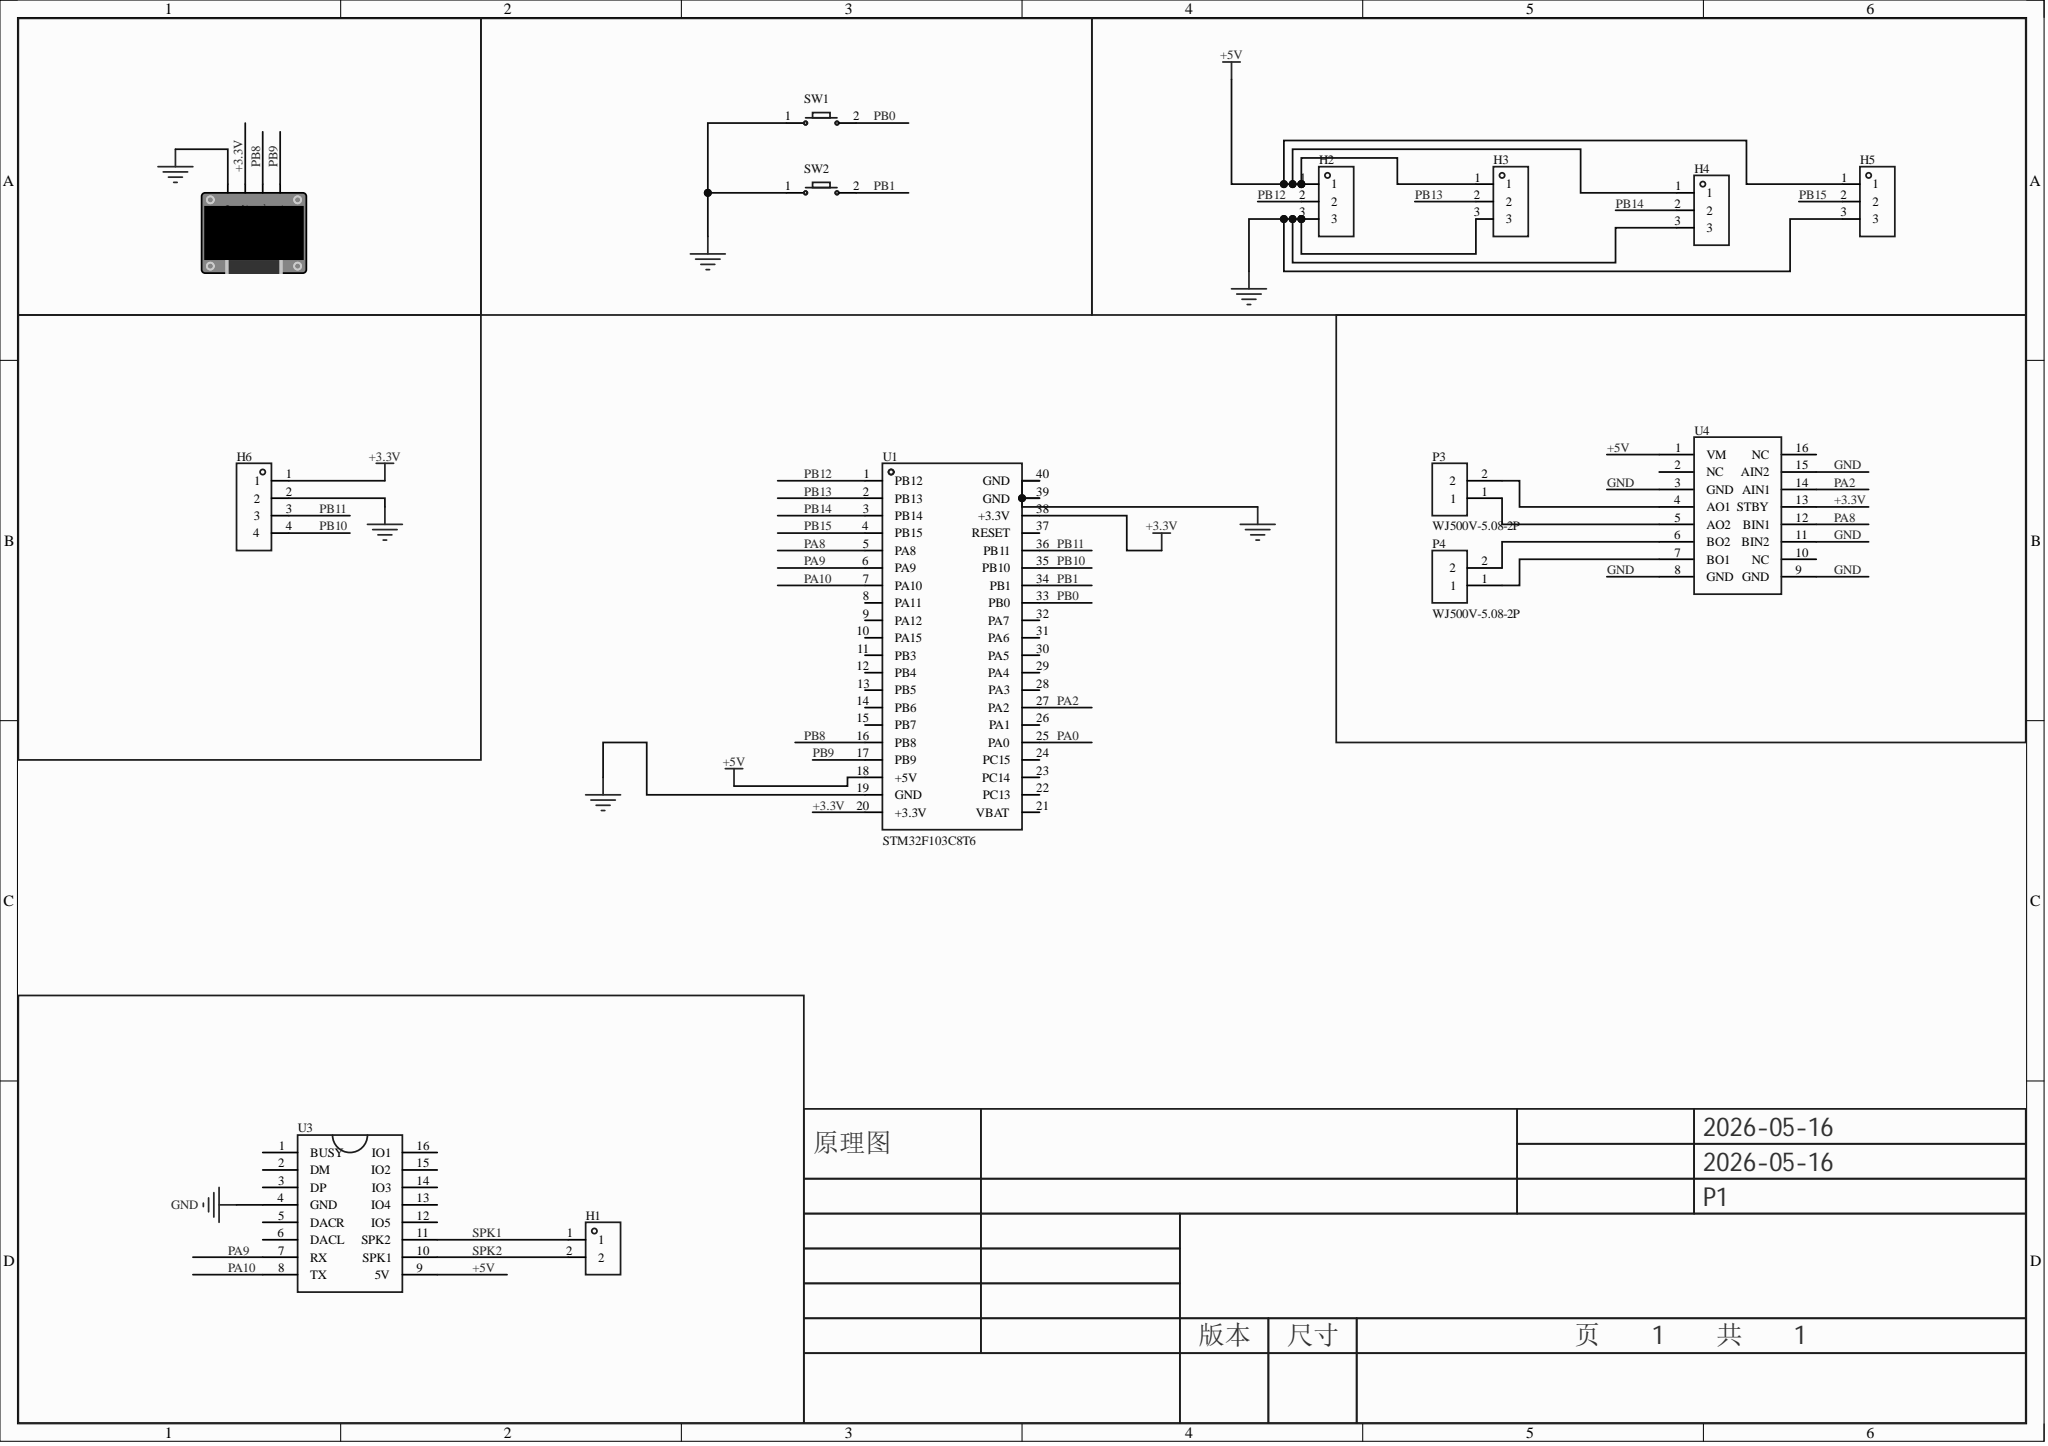Circuit board | Altium Designer | 14 parts | 23 nets
Bill of materials:
Comment,Description,Designator,Footprint,LibRef,Quantity
"HX PH254-01-02-Z-L11.5 male header connector","","H1","HDR-TH_2P-P2.54-V-M","HX PH254-01-02-Z-L11.5 male header connector","1"
"","","H2, H3, H4, H5","HDR-TH_3P-P2.54-V-F","HDR-F_2.54_1x3P","4"
"","","H6","HDR-TH_4P-P2.54-V-F","HDR-F_2.54_1x4P","1"
"","","OLED1","0.96OLED_4P","0.96OLED模块_4P","1"
"WJ500V-5.08-2P","","P3, P4","CONN-TH_2P-P5.00_WJ500V-5.08-2P","WJ500V-5.08-2P","2"
"","","SW1, SW2","Key_SMD_3x4x2","Key_SMD_3x4x2","2"
"STM32F103C8T6","","U1","CONN-TH_L53.3-W22.9_STM32F103C8T6-CARD","LCKFB-DKX-STM32F103C8T6","1"
"","","U3","MY2490-16P","MY2490-16PMP3语言播放","1"
"","","U4","DRV8833","DRV8833","1"
Netlist (Protel format):
[
H1
HDR-TH_2P-P2.54-V-M
HX PH254-01-02-Z-L11.5 male header connector



]
[
H2
HDR-TH_3P-P2.54-V-F




]
[
H3
HDR-TH_3P-P2.54-V-F




]
[
H4
HDR-TH_3P-P2.54-V-F




]
[
H5
HDR-TH_3P-P2.54-V-F




]
[
H6
HDR-TH_4P-P2.54-V-F




]
[
OLED1
0.96OLED_4P




]
[
P3
CONN-TH_2P-P5.00_WJ500V-5.08-2P
WJ500V-5.08-2P



]
[
P4
CONN-TH_2P-P5.00_WJ500V-5.08-2P
WJ500V-5.08-2P



]
[
SW1
Key_SMD_3x4x2




]
[
SW2
Key_SMD_3x4x2




]
[
U1
CONN-TH_L53.3-W22.9_STM32F103C8T6-CARD
STM32F103C8T6



]
[
U3
MY2490-16P




]
[
U4
DRV8833




]
(
SPK2
H1-2
U3-10
)
(
SPK1
H1-1
U3-11
)
(
PB15
H5-2
U1-4
)
(
PB14
H4-2
U1-3
)
(
PB13
H3-2
U1-2
)
(
PB12
H2-2
U1-1
)
(
PB11
H6-3
U1-36
)
(
PB10
H6-4
U1-35
)
(
PB9
OLED1-4
U1-17
)
(
PB8
OLED1-3
U1-16
)
(
PB1
SW2-2
U1-34
)
(
PB0
SW1-2
U1-33
)
(
PA10
U1-7
U3-8
)
(
PA9
U1-6
U3-7
)
(
PA8
U1-5
U4-12
)
(
PA2
U1-27
U4-14
)
(
NetP4_2
P4-2
U4-6
)
(
NetP4_1
P4-1
U4-7
)
(
NetP3_2
P3-2
U4-4
)
(
NetP3_1
P3-1
U4-5
)
(
GND
H2-3
H3-3
H4-3
H5-3
H6-2
OLED1-1
SW1-1
SW2-1
U1-19
U1-39
U1-40
U3-4
U4-3
U4-8
U4-9
U4-11
U4-15
)
(
+5V
H2-1
H3-1
H4-1
H5-1
U1-18
U3-9
U4-1
)
(
+3.3V
H6-1
OLED1-2
U1-20
U1-38
U4-13
)